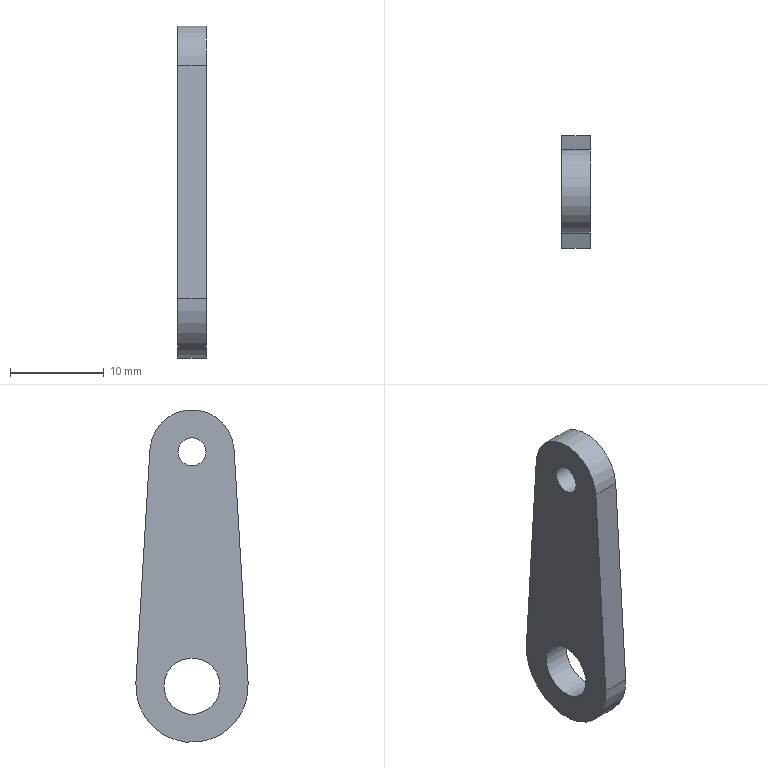Part | STEP file | 2-09.1 | 1 solid | 8 faces | box 3 x 12 x 35.5 mm | volume 947.961 mm3 | plane 4 | cylinder 4 | commonest cylinder face diameters 3 x1 6 x1 9 x1 12 x1
STEP:
#1=CARTESIAN_POINT('',(0.,0.,0.));
#2=DIRECTION('',(0.,0.,1.));
#3=DIRECTION('',(1.,0.,0.));
#4=AXIS2_PLACEMENT_3D('',#1,#2,#3);
#5=CARTESIAN_POINT('',(0.,4.492,0.27));
#6=VERTEX_POINT('',#5);
#7=CARTESIAN_POINT('',(0.,-4.492,0.27));
#8=VERTEX_POINT('',#7);
#9=CARTESIAN_POINT('',(0.,0.,0.));
#10=DIRECTION('',(1.,0.,0.));
#11=DIRECTION('',(0.,0.9982,0.06));
#12=AXIS2_PLACEMENT_3D('',#9,#10,#11);
#13=CIRCLE('',#12,4.5);
#14=CARTESIAN_POINT('',(0.,11.379,-13.25));
#15=DIRECTION('',(1.,0.,0.));
#16=DIRECTION('',(0.,1.,0.));
#17=AXIS2_PLACEMENT_3D('',#14,#15,#16);
#18=PLANE('',#17);
#19=CARTESIAN_POINT('',(-11.379,13.25));
#20=DIRECTION('',(0.9982,0.06));
#21=AXIS2_PLACEMENT_2D('',#19,#20);
#22=CIRCLE('',#21,4.5);
#23=(GEOMETRIC_REPRESENTATION_CONTEXT(2)PARAMETRIC_REPRESENTATION_CONTEXT()REPRESENTATION_CONTEXT('',''));
#24=DEFINITIONAL_REPRESENTATION('',(#22),#23);
#25=PCURVE('',#18,#24);
#26=CARTESIAN_POINT('',(0.,0.,0.));
#27=DIRECTION('',(-1.,0.,0.));
#28=DIRECTION('',(0.,0.9982,0.06));
#29=AXIS2_PLACEMENT_3D('',#26,#27,#28);
#30=CYLINDRICAL_SURFACE('',#29,4.5);
#31=CARTESIAN_POINT('',(6.283,0.));
#32=DIRECTION('',(-1.,0.));
#33=VECTOR('',#32,1.);
#34=LINE('',#31,#33);
#35=(GEOMETRIC_REPRESENTATION_CONTEXT(2)PARAMETRIC_REPRESENTATION_CONTEXT()REPRESENTATION_CONTEXT('',''));
#36=DEFINITIONAL_REPRESENTATION('',(#34),#35);
#37=PCURVE('',#30,#36);
#38=SURFACE_CURVE('',#13,(#25,#37),.PCURVE_S1.);
#39=EDGE_CURVE('',#6,#8,#38,.T.);
#40=ORIENTED_EDGE('',*,*,#39,.T.);
#41=CARTESIAN_POINT('',(0.,-5.989,-24.64));
#42=VERTEX_POINT('',#41);
#43=CARTESIAN_POINT('',(0.,-4.492,0.27));
#44=DIRECTION('',(0.,-0.06,-0.9982));
#45=VECTOR('',#44,1.);
#46=LINE('',#43,#45);
#47=CARTESIAN_POINT('',(-15.87,13.52));
#48=DIRECTION('',(-0.06,-0.9982));
#49=VECTOR('',#48,1.);
#50=LINE('',#47,#49);
#51=(GEOMETRIC_REPRESENTATION_CONTEXT(2)PARAMETRIC_REPRESENTATION_CONTEXT()REPRESENTATION_CONTEXT('',''));
#52=DEFINITIONAL_REPRESENTATION('',(#50),#51);
#53=PCURVE('',#18,#52);
#54=CARTESIAN_POINT('',(-1.5,-5.241,-12.185));
#55=DIRECTION('',(0.,0.9982,-0.06));
#56=DIRECTION('',(0.,-0.06,-0.9982));
#57=AXIS2_PLACEMENT_3D('',#54,#55,#56);
#58=PLANE('',#57);
#59=CARTESIAN_POINT('',(-12.477,-1.5));
#60=DIRECTION('',(1.,0.));
#61=VECTOR('',#60,1.);
#62=LINE('',#59,#61);
#63=(GEOMETRIC_REPRESENTATION_CONTEXT(2)PARAMETRIC_REPRESENTATION_CONTEXT()REPRESENTATION_CONTEXT('',''));
#64=DEFINITIONAL_REPRESENTATION('',(#62),#63);
#65=PCURVE('',#58,#64);
#66=SURFACE_CURVE('',#46,(#53,#65),.PCURVE_S1.);
#67=EDGE_CURVE('',#8,#42,#66,.T.);
#68=ORIENTED_EDGE('',*,*,#67,.T.);
#69=CARTESIAN_POINT('',(0.,5.989,-24.64));
#70=VERTEX_POINT('',#69);
#71=CARTESIAN_POINT('',(0.,0.,-25.));
#72=DIRECTION('',(1.,0.,0.));
#73=DIRECTION('',(0.,-0.9982,0.06));
#74=AXIS2_PLACEMENT_3D('',#71,#72,#73);
#75=CIRCLE('',#74,6.);
#76=CARTESIAN_POINT('',(-11.379,-11.75));
#77=DIRECTION('',(-0.9982,0.06));
#78=AXIS2_PLACEMENT_2D('',#76,#77);
#79=CIRCLE('',#78,6.);
#80=(GEOMETRIC_REPRESENTATION_CONTEXT(2)PARAMETRIC_REPRESENTATION_CONTEXT()REPRESENTATION_CONTEXT('',''));
#81=DEFINITIONAL_REPRESENTATION('',(#79),#80);
#82=PCURVE('',#18,#81);
#83=CARTESIAN_POINT('',(0.,0.,-25.));
#84=DIRECTION('',(-1.,0.,0.));
#85=DIRECTION('',(0.,-0.9982,0.06));
#86=AXIS2_PLACEMENT_3D('',#83,#84,#85);
#87=CYLINDRICAL_SURFACE('',#86,6.);
#88=CARTESIAN_POINT('',(6.283,0.));
#89=DIRECTION('',(-1.,0.));
#90=VECTOR('',#89,1.);
#91=LINE('',#88,#90);
#92=(GEOMETRIC_REPRESENTATION_CONTEXT(2)PARAMETRIC_REPRESENTATION_CONTEXT()REPRESENTATION_CONTEXT('',''));
#93=DEFINITIONAL_REPRESENTATION('',(#91),#92);
#94=PCURVE('',#87,#93);
#95=SURFACE_CURVE('',#75,(#82,#94),.PCURVE_S1.);
#96=EDGE_CURVE('',#42,#70,#95,.T.);
#97=ORIENTED_EDGE('',*,*,#96,.T.);
#98=CARTESIAN_POINT('',(0.,5.989,-24.64));
#99=DIRECTION('',(0.,-0.06,0.9982));
#100=VECTOR('',#99,1.);
#101=LINE('',#98,#100);
#102=CARTESIAN_POINT('',(-5.389,-11.39));
#103=DIRECTION('',(-0.06,0.9982));
#104=VECTOR('',#103,1.);
#105=LINE('',#102,#104);
#106=(GEOMETRIC_REPRESENTATION_CONTEXT(2)PARAMETRIC_REPRESENTATION_CONTEXT()REPRESENTATION_CONTEXT('',''));
#107=DEFINITIONAL_REPRESENTATION('',(#105),#106);
#108=PCURVE('',#18,#107);
#109=CARTESIAN_POINT('',(-1.5,5.241,-12.185));
#110=DIRECTION('',(0.,-0.9982,-0.06));
#111=DIRECTION('',(0.,-0.06,0.9982));
#112=AXIS2_PLACEMENT_3D('',#109,#110,#111);
#113=PLANE('',#112);
#114=CARTESIAN_POINT('',(-12.477,-1.5));
#115=DIRECTION('',(1.,0.));
#116=VECTOR('',#115,1.);
#117=LINE('',#114,#116);
#118=(GEOMETRIC_REPRESENTATION_CONTEXT(2)PARAMETRIC_REPRESENTATION_CONTEXT()REPRESENTATION_CONTEXT('',''));
#119=DEFINITIONAL_REPRESENTATION('',(#117),#118);
#120=PCURVE('',#113,#119);
#121=SURFACE_CURVE('',#101,(#108,#120),.PCURVE_S1.);
#122=EDGE_CURVE('',#70,#6,#121,.T.);
#123=ORIENTED_EDGE('',*,*,#122,.T.);
#124=EDGE_LOOP('',(#40,#68,#97,#123));
#125=FACE_BOUND('',#124,.T.);
#126=CARTESIAN_POINT('',(0.,1.5,0.));
#127=VERTEX_POINT('',#126);
#128=CARTESIAN_POINT('',(0.,0.,0.));
#129=DIRECTION('',(-1.,0.,0.));
#130=DIRECTION('',(0.,1.,0.));
#131=AXIS2_PLACEMENT_3D('',#128,#129,#130);
#132=CIRCLE('',#131,1.5);
#133=CARTESIAN_POINT('',(-9.879,13.25));
#134=CARTESIAN_POINT('',(-9.879,10.652));
#135=CARTESIAN_POINT('',(-12.129,11.951));
#136=CARTESIAN_POINT('',(-14.379,13.25));
#137=CARTESIAN_POINT('',(-12.129,14.549));
#138=CARTESIAN_POINT('',(-9.879,15.848));
#139=CARTESIAN_POINT('',(-9.879,13.25));
#140=(BOUNDED_CURVE()B_SPLINE_CURVE(2,(#133,#134,#135,#136,#137,#138,#139),.UNSPECIFIED.,.T.,.F.)B_SPLINE_CURVE_WITH_KNOTS((1,2,2,2,2,1),(-2.094,0.,2.094,4.189,6.283,8.378),.UNSPECIFIED.)CURVE()GEOMETRIC_REPRESENTATION_ITEM()RATIONAL_B_SPLINE_CURVE((1.,0.5,1.,0.5,1.,0.5,1.))REPRESENTATION_ITEM(''));
#141=(GEOMETRIC_REPRESENTATION_CONTEXT(2)PARAMETRIC_REPRESENTATION_CONTEXT()REPRESENTATION_CONTEXT('',''));
#142=DEFINITIONAL_REPRESENTATION('',(#140),#141);
#143=PCURVE('',#18,#142);
#144=CARTESIAN_POINT('',(0.,0.,0.));
#145=DIRECTION('',(-1.,0.,0.));
#146=DIRECTION('',(0.,1.,0.));
#147=AXIS2_PLACEMENT_3D('',#144,#145,#146);
#148=CYLINDRICAL_SURFACE('',#147,1.5);
#149=CARTESIAN_POINT('',(0.,0.));
#150=DIRECTION('',(1.,0.));
#151=VECTOR('',#150,1.);
#152=LINE('',#149,#151);
#153=(GEOMETRIC_REPRESENTATION_CONTEXT(2)PARAMETRIC_REPRESENTATION_CONTEXT()REPRESENTATION_CONTEXT('',''));
#154=DEFINITIONAL_REPRESENTATION('',(#152),#153);
#155=PCURVE('',#148,#154);
#156=SURFACE_CURVE('',#132,(#143,#155),.PCURVE_S1.);
#157=EDGE_CURVE('',#127,#127,#156,.T.);
#158=ORIENTED_EDGE('',*,*,#157,.T.);
#159=EDGE_LOOP('',(#158));
#160=FACE_BOUND('',#159,.T.);
#161=CARTESIAN_POINT('',(0.,3.,-25.));
#162=VERTEX_POINT('',#161);
#163=CARTESIAN_POINT('',(0.,0.,-25.));
#164=DIRECTION('',(-1.,0.,0.));
#165=DIRECTION('',(0.,1.,0.));
#166=AXIS2_PLACEMENT_3D('',#163,#164,#165);
#167=CIRCLE('',#166,3.);
#168=CARTESIAN_POINT('',(-8.379,-11.75));
#169=CARTESIAN_POINT('',(-8.379,-16.946));
#170=CARTESIAN_POINT('',(-12.879,-14.348));
#171=CARTESIAN_POINT('',(-17.379,-11.75));
#172=CARTESIAN_POINT('',(-12.879,-9.152));
#173=CARTESIAN_POINT('',(-8.379,-6.554));
#174=CARTESIAN_POINT('',(-8.379,-11.75));
#175=(BOUNDED_CURVE()B_SPLINE_CURVE(2,(#168,#169,#170,#171,#172,#173,#174),.UNSPECIFIED.,.T.,.F.)B_SPLINE_CURVE_WITH_KNOTS((1,2,2,2,2,1),(-2.094,0.,2.094,4.189,6.283,8.378),.UNSPECIFIED.)CURVE()GEOMETRIC_REPRESENTATION_ITEM()RATIONAL_B_SPLINE_CURVE((1.,0.5,1.,0.5,1.,0.5,1.))REPRESENTATION_ITEM(''));
#176=(GEOMETRIC_REPRESENTATION_CONTEXT(2)PARAMETRIC_REPRESENTATION_CONTEXT()REPRESENTATION_CONTEXT('',''));
#177=DEFINITIONAL_REPRESENTATION('',(#175),#176);
#178=PCURVE('',#18,#177);
#179=CARTESIAN_POINT('',(0.,0.,-25.));
#180=DIRECTION('',(-1.,0.,0.));
#181=DIRECTION('',(0.,1.,0.));
#182=AXIS2_PLACEMENT_3D('',#179,#180,#181);
#183=CYLINDRICAL_SURFACE('',#182,3.);
#184=CARTESIAN_POINT('',(0.,0.));
#185=DIRECTION('',(1.,0.));
#186=VECTOR('',#185,1.);
#187=LINE('',#184,#186);
#188=(GEOMETRIC_REPRESENTATION_CONTEXT(2)PARAMETRIC_REPRESENTATION_CONTEXT()REPRESENTATION_CONTEXT('',''));
#189=DEFINITIONAL_REPRESENTATION('',(#187),#188);
#190=PCURVE('',#183,#189);
#191=SURFACE_CURVE('',#167,(#178,#190),.PCURVE_S1.);
#192=EDGE_CURVE('',#162,#162,#191,.T.);
#193=ORIENTED_EDGE('',*,*,#192,.T.);
#194=EDGE_LOOP('',(#193));
#195=FACE_BOUND('',#194,.T.);
#196=ADVANCED_FACE('',(#125,#160,#195),#18,.T.);
#197=CARTESIAN_POINT('',(-3.,4.492,0.27));
#198=VERTEX_POINT('',#197);
#199=CARTESIAN_POINT('',(-3.,-4.492,0.27));
#200=VERTEX_POINT('',#199);
#201=CARTESIAN_POINT('',(-3.,0.,0.));
#202=DIRECTION('',(1.,0.,0.));
#203=DIRECTION('',(0.,0.9982,0.06));
#204=AXIS2_PLACEMENT_3D('',#201,#202,#203);
#205=CIRCLE('',#204,4.5);
#206=CARTESIAN_POINT('',(-3.,11.379,-13.25));
#207=DIRECTION('',(1.,0.,0.));
#208=DIRECTION('',(0.,1.,0.));
#209=AXIS2_PLACEMENT_3D('',#206,#207,#208);
#210=PLANE('',#209);
#211=CARTESIAN_POINT('',(-11.379,13.25));
#212=DIRECTION('',(0.9982,0.06));
#213=AXIS2_PLACEMENT_2D('',#211,#212);
#214=CIRCLE('',#213,4.5);
#215=(GEOMETRIC_REPRESENTATION_CONTEXT(2)PARAMETRIC_REPRESENTATION_CONTEXT()REPRESENTATION_CONTEXT('',''));
#216=DEFINITIONAL_REPRESENTATION('',(#214),#215);
#217=PCURVE('',#210,#216);
#218=CARTESIAN_POINT('',(6.283,3.));
#219=DIRECTION('',(-1.,0.));
#220=VECTOR('',#219,1.);
#221=LINE('',#218,#220);
#222=(GEOMETRIC_REPRESENTATION_CONTEXT(2)PARAMETRIC_REPRESENTATION_CONTEXT()REPRESENTATION_CONTEXT('',''));
#223=DEFINITIONAL_REPRESENTATION('',(#221),#222);
#224=PCURVE('',#30,#223);
#225=SURFACE_CURVE('',#205,(#217,#224),.PCURVE_S1.);
#226=EDGE_CURVE('',#198,#200,#225,.T.);
#227=ORIENTED_EDGE('',*,*,#226,.T.);
#228=CARTESIAN_POINT('',(-3.,-5.989,-24.64));
#229=VERTEX_POINT('',#228);
#230=CARTESIAN_POINT('',(-3.,-4.492,0.27));
#231=DIRECTION('',(0.,-0.06,-0.9982));
#232=VECTOR('',#231,1.);
#233=LINE('',#230,#232);
#234=CARTESIAN_POINT('',(-15.87,13.52));
#235=DIRECTION('',(-0.06,-0.9982));
#236=VECTOR('',#235,1.);
#237=LINE('',#234,#236);
#238=(GEOMETRIC_REPRESENTATION_CONTEXT(2)PARAMETRIC_REPRESENTATION_CONTEXT()REPRESENTATION_CONTEXT('',''));
#239=DEFINITIONAL_REPRESENTATION('',(#237),#238);
#240=PCURVE('',#210,#239);
#241=CARTESIAN_POINT('',(-12.477,1.5));
#242=DIRECTION('',(1.,0.));
#243=VECTOR('',#242,1.);
#244=LINE('',#241,#243);
#245=(GEOMETRIC_REPRESENTATION_CONTEXT(2)PARAMETRIC_REPRESENTATION_CONTEXT()REPRESENTATION_CONTEXT('',''));
#246=DEFINITIONAL_REPRESENTATION('',(#244),#245);
#247=PCURVE('',#58,#246);
#248=SURFACE_CURVE('',#233,(#240,#247),.PCURVE_S1.);
#249=EDGE_CURVE('',#200,#229,#248,.T.);
#250=ORIENTED_EDGE('',*,*,#249,.T.);
#251=CARTESIAN_POINT('',(-3.,5.989,-24.64));
#252=VERTEX_POINT('',#251);
#253=CARTESIAN_POINT('',(-3.,0.,-25.));
#254=DIRECTION('',(1.,0.,0.));
#255=DIRECTION('',(0.,-0.9982,0.06));
#256=AXIS2_PLACEMENT_3D('',#253,#254,#255);
#257=CIRCLE('',#256,6.);
#258=CARTESIAN_POINT('',(-11.379,-11.75));
#259=DIRECTION('',(-0.9982,0.06));
#260=AXIS2_PLACEMENT_2D('',#258,#259);
#261=CIRCLE('',#260,6.);
#262=(GEOMETRIC_REPRESENTATION_CONTEXT(2)PARAMETRIC_REPRESENTATION_CONTEXT()REPRESENTATION_CONTEXT('',''));
#263=DEFINITIONAL_REPRESENTATION('',(#261),#262);
#264=PCURVE('',#210,#263);
#265=CARTESIAN_POINT('',(6.283,3.));
#266=DIRECTION('',(-1.,0.));
#267=VECTOR('',#266,1.);
#268=LINE('',#265,#267);
#269=(GEOMETRIC_REPRESENTATION_CONTEXT(2)PARAMETRIC_REPRESENTATION_CONTEXT()REPRESENTATION_CONTEXT('',''));
#270=DEFINITIONAL_REPRESENTATION('',(#268),#269);
#271=PCURVE('',#87,#270);
#272=SURFACE_CURVE('',#257,(#264,#271),.PCURVE_S1.);
#273=EDGE_CURVE('',#229,#252,#272,.T.);
#274=ORIENTED_EDGE('',*,*,#273,.T.);
#275=CARTESIAN_POINT('',(-3.,5.989,-24.64));
#276=DIRECTION('',(0.,-0.06,0.9982));
#277=VECTOR('',#276,1.);
#278=LINE('',#275,#277);
#279=CARTESIAN_POINT('',(-5.389,-11.39));
#280=DIRECTION('',(-0.06,0.9982));
#281=VECTOR('',#280,1.);
#282=LINE('',#279,#281);
#283=(GEOMETRIC_REPRESENTATION_CONTEXT(2)PARAMETRIC_REPRESENTATION_CONTEXT()REPRESENTATION_CONTEXT('',''));
#284=DEFINITIONAL_REPRESENTATION('',(#282),#283);
#285=PCURVE('',#210,#284);
#286=CARTESIAN_POINT('',(-12.477,1.5));
#287=DIRECTION('',(1.,0.));
#288=VECTOR('',#287,1.);
#289=LINE('',#286,#288);
#290=(GEOMETRIC_REPRESENTATION_CONTEXT(2)PARAMETRIC_REPRESENTATION_CONTEXT()REPRESENTATION_CONTEXT('',''));
#291=DEFINITIONAL_REPRESENTATION('',(#289),#290);
#292=PCURVE('',#113,#291);
#293=SURFACE_CURVE('',#278,(#285,#292),.PCURVE_S1.);
#294=EDGE_CURVE('',#252,#198,#293,.T.);
#295=ORIENTED_EDGE('',*,*,#294,.T.);
#296=EDGE_LOOP('',(#227,#250,#274,#295));
#297=FACE_BOUND('',#296,.F.);
#298=CARTESIAN_POINT('',(-3.,1.5,0.));
#299=VERTEX_POINT('',#298);
#300=CARTESIAN_POINT('',(-3.,0.,0.));
#301=DIRECTION('',(-1.,0.,0.));
#302=DIRECTION('',(0.,1.,0.));
#303=AXIS2_PLACEMENT_3D('',#300,#301,#302);
#304=CIRCLE('',#303,1.5);
#305=CARTESIAN_POINT('',(-9.879,13.25));
#306=CARTESIAN_POINT('',(-9.879,10.652));
#307=CARTESIAN_POINT('',(-12.129,11.951));
#308=CARTESIAN_POINT('',(-14.379,13.25));
#309=CARTESIAN_POINT('',(-12.129,14.549));
#310=CARTESIAN_POINT('',(-9.879,15.848));
#311=CARTESIAN_POINT('',(-9.879,13.25));
#312=(BOUNDED_CURVE()B_SPLINE_CURVE(2,(#305,#306,#307,#308,#309,#310,#311),.UNSPECIFIED.,.T.,.F.)B_SPLINE_CURVE_WITH_KNOTS((1,2,2,2,2,1),(-2.094,0.,2.094,4.189,6.283,8.378),.UNSPECIFIED.)CURVE()GEOMETRIC_REPRESENTATION_ITEM()RATIONAL_B_SPLINE_CURVE((1.,0.5,1.,0.5,1.,0.5,1.))REPRESENTATION_ITEM(''));
#313=(GEOMETRIC_REPRESENTATION_CONTEXT(2)PARAMETRIC_REPRESENTATION_CONTEXT()REPRESENTATION_CONTEXT('',''));
#314=DEFINITIONAL_REPRESENTATION('',(#312),#313);
#315=PCURVE('',#210,#314);
#316=CARTESIAN_POINT('',(0.,3.));
#317=DIRECTION('',(1.,0.));
#318=VECTOR('',#317,1.);
#319=LINE('',#316,#318);
#320=(GEOMETRIC_REPRESENTATION_CONTEXT(2)PARAMETRIC_REPRESENTATION_CONTEXT()REPRESENTATION_CONTEXT('',''));
#321=DEFINITIONAL_REPRESENTATION('',(#319),#320);
#322=PCURVE('',#148,#321);
#323=SURFACE_CURVE('',#304,(#315,#322),.PCURVE_S1.);
#324=EDGE_CURVE('',#299,#299,#323,.T.);
#325=ORIENTED_EDGE('',*,*,#324,.T.);
#326=EDGE_LOOP('',(#325));
#327=FACE_BOUND('',#326,.F.);
#328=CARTESIAN_POINT('',(-3.,3.,-25.));
#329=VERTEX_POINT('',#328);
#330=CARTESIAN_POINT('',(-3.,0.,-25.));
#331=DIRECTION('',(-1.,0.,0.));
#332=DIRECTION('',(0.,1.,0.));
#333=AXIS2_PLACEMENT_3D('',#330,#331,#332);
#334=CIRCLE('',#333,3.);
#335=CARTESIAN_POINT('',(-8.379,-11.75));
#336=CARTESIAN_POINT('',(-8.379,-16.946));
#337=CARTESIAN_POINT('',(-12.879,-14.348));
#338=CARTESIAN_POINT('',(-17.379,-11.75));
#339=CARTESIAN_POINT('',(-12.879,-9.152));
#340=CARTESIAN_POINT('',(-8.379,-6.554));
#341=CARTESIAN_POINT('',(-8.379,-11.75));
#342=(BOUNDED_CURVE()B_SPLINE_CURVE(2,(#335,#336,#337,#338,#339,#340,#341),.UNSPECIFIED.,.T.,.F.)B_SPLINE_CURVE_WITH_KNOTS((1,2,2,2,2,1),(-2.094,0.,2.094,4.189,6.283,8.378),.UNSPECIFIED.)CURVE()GEOMETRIC_REPRESENTATION_ITEM()RATIONAL_B_SPLINE_CURVE((1.,0.5,1.,0.5,1.,0.5,1.))REPRESENTATION_ITEM(''));
#343=(GEOMETRIC_REPRESENTATION_CONTEXT(2)PARAMETRIC_REPRESENTATION_CONTEXT()REPRESENTATION_CONTEXT('',''));
#344=DEFINITIONAL_REPRESENTATION('',(#342),#343);
#345=PCURVE('',#210,#344);
#346=CARTESIAN_POINT('',(0.,3.));
#347=DIRECTION('',(1.,0.));
#348=VECTOR('',#347,1.);
#349=LINE('',#346,#348);
#350=(GEOMETRIC_REPRESENTATION_CONTEXT(2)PARAMETRIC_REPRESENTATION_CONTEXT()REPRESENTATION_CONTEXT('',''));
#351=DEFINITIONAL_REPRESENTATION('',(#349),#350);
#352=PCURVE('',#183,#351);
#353=SURFACE_CURVE('',#334,(#345,#352),.PCURVE_S1.);
#354=EDGE_CURVE('',#329,#329,#353,.T.);
#355=ORIENTED_EDGE('',*,*,#354,.T.);
#356=EDGE_LOOP('',(#355));
#357=FACE_BOUND('',#356,.F.);
#358=ADVANCED_FACE('',(#297,#327,#357),#210,.F.);
#359=CARTESIAN_POINT('',(0.,4.492,0.27));
#360=DIRECTION('',(-1.,0.,0.));
#361=VECTOR('',#360,1.);
#362=LINE('',#359,#361);
#363=CARTESIAN_POINT('',(6.283,0.));
#364=DIRECTION('',(0.,1.));
#365=VECTOR('',#364,1.);
#366=LINE('',#363,#365);
#367=(GEOMETRIC_REPRESENTATION_CONTEXT(2)PARAMETRIC_REPRESENTATION_CONTEXT()REPRESENTATION_CONTEXT('',''));
#368=DEFINITIONAL_REPRESENTATION('',(#366),#367);
#369=PCURVE('',#30,#368);
#370=CARTESIAN_POINT('',(12.477,-1.5));
#371=DIRECTION('',(0.,1.));
#372=VECTOR('',#371,1.);
#373=LINE('',#370,#372);
#374=(GEOMETRIC_REPRESENTATION_CONTEXT(2)PARAMETRIC_REPRESENTATION_CONTEXT()REPRESENTATION_CONTEXT('',''));
#375=DEFINITIONAL_REPRESENTATION('',(#373),#374);
#376=PCURVE('',#113,#375);
#377=SURFACE_CURVE('',#362,(#369,#376),.PCURVE_S1.);
#378=EDGE_CURVE('',#6,#198,#377,.T.);
#379=ORIENTED_EDGE('',*,*,#378,.T.);
#380=ORIENTED_EDGE('',*,*,#226,.T.);
#381=CARTESIAN_POINT('',(0.,-4.492,0.27));
#382=DIRECTION('',(-1.,0.,0.));
#383=VECTOR('',#382,1.);
#384=LINE('',#381,#383);
#385=CARTESIAN_POINT('',(3.262,0.));
#386=DIRECTION('',(0.,1.));
#387=VECTOR('',#386,1.);
#388=LINE('',#385,#387);
#389=(GEOMETRIC_REPRESENTATION_CONTEXT(2)PARAMETRIC_REPRESENTATION_CONTEXT()REPRESENTATION_CONTEXT('',''));
#390=DEFINITIONAL_REPRESENTATION('',(#388),#389);
#391=PCURVE('',#30,#390);
#392=CARTESIAN_POINT('',(-12.477,-1.5));
#393=DIRECTION('',(0.,1.));
#394=VECTOR('',#393,1.);
#395=LINE('',#392,#394);
#396=(GEOMETRIC_REPRESENTATION_CONTEXT(2)PARAMETRIC_REPRESENTATION_CONTEXT()REPRESENTATION_CONTEXT('',''));
#397=DEFINITIONAL_REPRESENTATION('',(#395),#396);
#398=PCURVE('',#58,#397);
#399=SURFACE_CURVE('',#384,(#391,#398),.PCURVE_S1.);
#400=EDGE_CURVE('',#8,#200,#399,.T.);
#401=ORIENTED_EDGE('',*,*,#400,.F.);
#402=ORIENTED_EDGE('',*,*,#39,.F.);
#403=EDGE_LOOP('',(#379,#380,#401,#402));
#404=FACE_BOUND('',#403,.T.);
#405=ADVANCED_FACE('',(#404),#30,.T.);
#406=ORIENTED_EDGE('',*,*,#67,.T.);
#407=CARTESIAN_POINT('',(0.,-5.989,-24.64));
#408=DIRECTION('',(-1.,0.,0.));
#409=VECTOR('',#408,1.);
#410=LINE('',#407,#409);
#411=CARTESIAN_POINT('',(12.477,-1.5));
#412=DIRECTION('',(0.,1.));
#413=VECTOR('',#412,1.);
#414=LINE('',#411,#413);
#415=(GEOMETRIC_REPRESENTATION_CONTEXT(2)PARAMETRIC_REPRESENTATION_CONTEXT()REPRESENTATION_CONTEXT('',''));
#416=DEFINITIONAL_REPRESENTATION('',(#414),#415);
#417=PCURVE('',#58,#416);
#418=CARTESIAN_POINT('',(6.283,0.));
#419=DIRECTION('',(0.,1.));
#420=VECTOR('',#419,1.);
#421=LINE('',#418,#420);
#422=(GEOMETRIC_REPRESENTATION_CONTEXT(2)PARAMETRIC_REPRESENTATION_CONTEXT()REPRESENTATION_CONTEXT('',''));
#423=DEFINITIONAL_REPRESENTATION('',(#421),#422);
#424=PCURVE('',#87,#423);
#425=SURFACE_CURVE('',#410,(#417,#424),.PCURVE_S1.);
#426=EDGE_CURVE('',#42,#229,#425,.T.);
#427=ORIENTED_EDGE('',*,*,#426,.T.);
#428=ORIENTED_EDGE('',*,*,#249,.F.);
#429=ORIENTED_EDGE('',*,*,#400,.F.);
#430=EDGE_LOOP('',(#406,#427,#428,#429));
#431=FACE_BOUND('',#430,.F.);
#432=ADVANCED_FACE('',(#431),#58,.F.);
#433=ORIENTED_EDGE('',*,*,#426,.T.);
#434=ORIENTED_EDGE('',*,*,#273,.T.);
#435=CARTESIAN_POINT('',(0.,5.989,-24.64));
#436=DIRECTION('',(-1.,0.,0.));
#437=VECTOR('',#436,1.);
#438=LINE('',#435,#437);
#439=CARTESIAN_POINT('',(3.022,0.));
#440=DIRECTION('',(0.,1.));
#441=VECTOR('',#440,1.);
#442=LINE('',#439,#441);
#443=(GEOMETRIC_REPRESENTATION_CONTEXT(2)PARAMETRIC_REPRESENTATION_CONTEXT()REPRESENTATION_CONTEXT('',''));
#444=DEFINITIONAL_REPRESENTATION('',(#442),#443);
#445=PCURVE('',#87,#444);
#446=CARTESIAN_POINT('',(-12.477,-1.5));
#447=DIRECTION('',(0.,1.));
#448=VECTOR('',#447,1.);
#449=LINE('',#446,#448);
#450=(GEOMETRIC_REPRESENTATION_CONTEXT(2)PARAMETRIC_REPRESENTATION_CONTEXT()REPRESENTATION_CONTEXT('',''));
#451=DEFINITIONAL_REPRESENTATION('',(#449),#450);
#452=PCURVE('',#113,#451);
#453=SURFACE_CURVE('',#438,(#445,#452),.PCURVE_S1.);
#454=EDGE_CURVE('',#70,#252,#453,.T.);
#455=ORIENTED_EDGE('',*,*,#454,.F.);
#456=ORIENTED_EDGE('',*,*,#96,.F.);
#457=EDGE_LOOP('',(#433,#434,#455,#456));
#458=FACE_BOUND('',#457,.T.);
#459=ADVANCED_FACE('',(#458),#87,.T.);
#460=ORIENTED_EDGE('',*,*,#122,.T.);
#461=ORIENTED_EDGE('',*,*,#378,.T.);
#462=ORIENTED_EDGE('',*,*,#294,.F.);
#463=ORIENTED_EDGE('',*,*,#454,.F.);
#464=EDGE_LOOP('',(#460,#461,#462,#463));
#465=FACE_BOUND('',#464,.F.);
#466=ADVANCED_FACE('',(#465),#113,.F.);
#467=ORIENTED_EDGE('',*,*,#157,.T.);
#468=CARTESIAN_POINT('',(0.,1.5,0.));
#469=DIRECTION('',(-1.,0.,0.));
#470=VECTOR('',#469,1.);
#471=LINE('',#468,#470);
#472=CARTESIAN_POINT('',(6.283,0.));
#473=DIRECTION('',(0.,1.));
#474=VECTOR('',#473,1.);
#475=LINE('',#472,#474);
#476=(GEOMETRIC_REPRESENTATION_CONTEXT(2)PARAMETRIC_REPRESENTATION_CONTEXT()REPRESENTATION_CONTEXT('',''));
#477=DEFINITIONAL_REPRESENTATION('',(#475),#476);
#478=PCURVE('',#148,#477);
#479=CARTESIAN_POINT('',(0.,0.));
#480=DIRECTION('',(0.,1.));
#481=VECTOR('',#480,1.);
#482=LINE('',#479,#481);
#483=(GEOMETRIC_REPRESENTATION_CONTEXT(2)PARAMETRIC_REPRESENTATION_CONTEXT()REPRESENTATION_CONTEXT('',''));
#484=DEFINITIONAL_REPRESENTATION('',(#482),#483);
#485=PCURVE('',#148,#484);
#486=SEAM_CURVE('',#471,(#478,#485),.PCURVE_S1.);
#487=EDGE_CURVE('',#127,#299,#486,.T.);
#488=ORIENTED_EDGE('',*,*,#487,.T.);
#489=ORIENTED_EDGE('',*,*,#324,.F.);
#490=ORIENTED_EDGE('',*,*,#487,.F.);
#491=EDGE_LOOP('',(#467,#488,#489,#490));
#492=FACE_BOUND('',#491,.F.);
#493=ADVANCED_FACE('',(#492),#148,.F.);
#494=ORIENTED_EDGE('',*,*,#192,.T.);
#495=CARTESIAN_POINT('',(0.,3.,-25.));
#496=DIRECTION('',(-1.,0.,0.));
#497=VECTOR('',#496,1.);
#498=LINE('',#495,#497);
#499=CARTESIAN_POINT('',(6.283,0.));
#500=DIRECTION('',(0.,1.));
#501=VECTOR('',#500,1.);
#502=LINE('',#499,#501);
#503=(GEOMETRIC_REPRESENTATION_CONTEXT(2)PARAMETRIC_REPRESENTATION_CONTEXT()REPRESENTATION_CONTEXT('',''));
#504=DEFINITIONAL_REPRESENTATION('',(#502),#503);
#505=PCURVE('',#183,#504);
#506=CARTESIAN_POINT('',(0.,0.));
#507=DIRECTION('',(0.,1.));
#508=VECTOR('',#507,1.);
#509=LINE('',#506,#508);
#510=(GEOMETRIC_REPRESENTATION_CONTEXT(2)PARAMETRIC_REPRESENTATION_CONTEXT()REPRESENTATION_CONTEXT('',''));
#511=DEFINITIONAL_REPRESENTATION('',(#509),#510);
#512=PCURVE('',#183,#511);
#513=SEAM_CURVE('',#498,(#505,#512),.PCURVE_S1.);
#514=EDGE_CURVE('',#162,#329,#513,.T.);
#515=ORIENTED_EDGE('',*,*,#514,.T.);
#516=ORIENTED_EDGE('',*,*,#354,.F.);
#517=ORIENTED_EDGE('',*,*,#514,.F.);
#518=EDGE_LOOP('',(#494,#515,#516,#517));
#519=FACE_BOUND('',#518,.F.);
#520=ADVANCED_FACE('',(#519),#183,.F.);
#521=CLOSED_SHELL('',(#196,#358,#405,#432,#459,#466,#493,#520));
#522=MANIFOLD_SOLID_BREP('',#521);
#523=(LENGTH_UNIT()NAMED_UNIT(*)SI_UNIT(.MILLI.,.METRE.));
#524=UNCERTAINTY_MEASURE_WITH_UNIT(LENGTH_MEASURE(0.0000001),#523,'','');
#525=(NAMED_UNIT(*)PLANE_ANGLE_UNIT()SI_UNIT($,.RADIAN.));
#526=(NAMED_UNIT(*)SI_UNIT($,.STERADIAN.)SOLID_ANGLE_UNIT());
#527=(GEOMETRIC_REPRESENTATION_CONTEXT(3)GLOBAL_UNCERTAINTY_ASSIGNED_CONTEXT((#524))GLOBAL_UNIT_ASSIGNED_CONTEXT((#523,#525,#526))REPRESENTATION_CONTEXT('',''));
#528=ADVANCED_BREP_SHAPE_REPRESENTATION('',(#4,#522),#527);